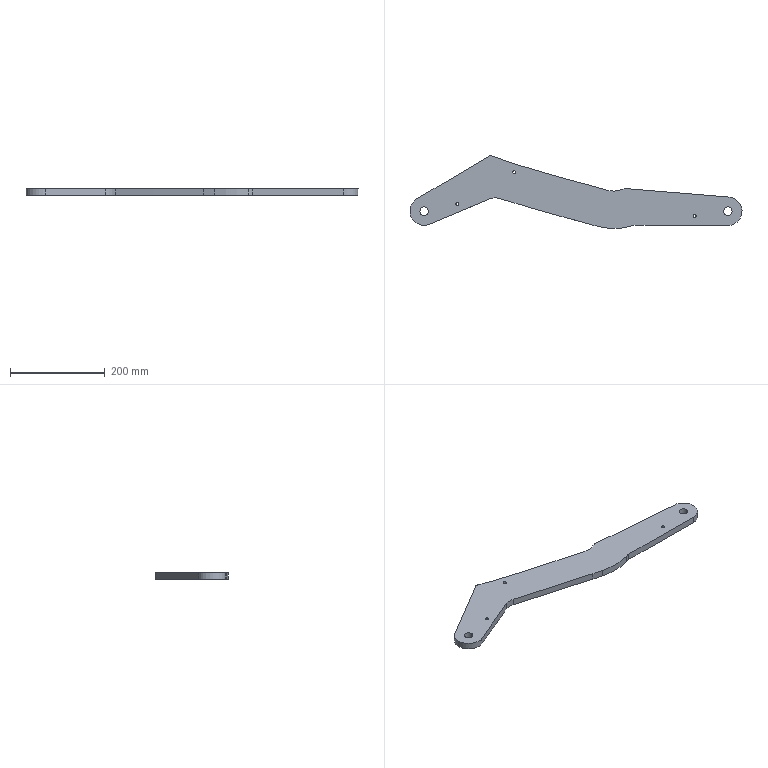CAM job | NX | 3-axis milling, drilling | part box 700 x 153.975 x 14 mm | stock box 720 x 175 x 17 mm
Tools:
number,name,description,diameter,corner_radius,flute_length,length,flutes
0,D20R0,Milling Tool-5 Parameters,20.0,0.0,50.0,75.0,2
0,D12,Drilling Tool,12.0,0.0,35.0,50.0,2
0,D0.1,Milling Tool-5 Parameters,0.1,0.0,50.0,75.0,2
0,D18,Drilling Tool,18.0,0.0,35.0,50.0,2
0,D6.35,Drilling Tool,6.35,0.0,35.0,50.0,2
0,D16R3,Milling Tool-5 Parameters,16.0,3.0,50.0,75.0,2
Operations:
program,operation,operation_type,tool,method,geometry_group,spindle_rpm,surface_speed,feed_per_tooth,feed_cut,feed_plunge,cut_length_mm,path_length_mm,cut_time_min,machine_time_min
XFK07-1,CAVITY_MILL,CavityMilling,D20R0,METHOD,MCS_MILL,4500.0,282.0,0.3889,3500.0,100.0,34310.772,36009.301,9.803,9.973
XFK07-2,CAVITY_MILL_COPY_1,CavityMilling,D20R0,METHOD,MCS_MILL,4500.0,282.0,0.3889,3500.0,100.0,23399.459,25203.819,6.686,6.866
XFK07-3,SPOT_FACING_COPY,Operation,D12,METHOD,WORKPIECE,0.0,0.0,0.0,250.0,0.0,12.0,870.028,0.048,0.1338
XFK07-4,ZLEVEL_PROFILE,ZLevelMilling,D20R0,METHOD,WORKPIECE,4500.0,282.0,0.3333,3000.0,100.0,6400.053,6616.053,2.133,2.155
XFK07-5,CONTOUR_TEXT,SurfaceContour,D0.1,METHOD,WORKPIECE,2000.0,0.0,0.25,1000.0,100.0,271.117,1151.601,0.2711,0.3592
XFK07-6,SPOT_FACING,Operation,D18,METHOD,WORKPIECE,0.0,0.0,0.0,250.0,0.0,12.0,876.028,0.048,0.1344
XFK07-7,SPOT_FACING_1,Operation,D6.35,METHOD,WORKPIECE,0.0,0.0,0.0,250.0,0.0,18.0,782.592,0.072,0.1485
XFK07-8,ZLEVEL_PROFILE_COPY_COPY,ZLevelMilling,D16R3,METHOD,WORKPIECE_COPY,4500.0,282.0,0.3333,3000.0,100.0,80738.354,84277.97,26.913,27.267